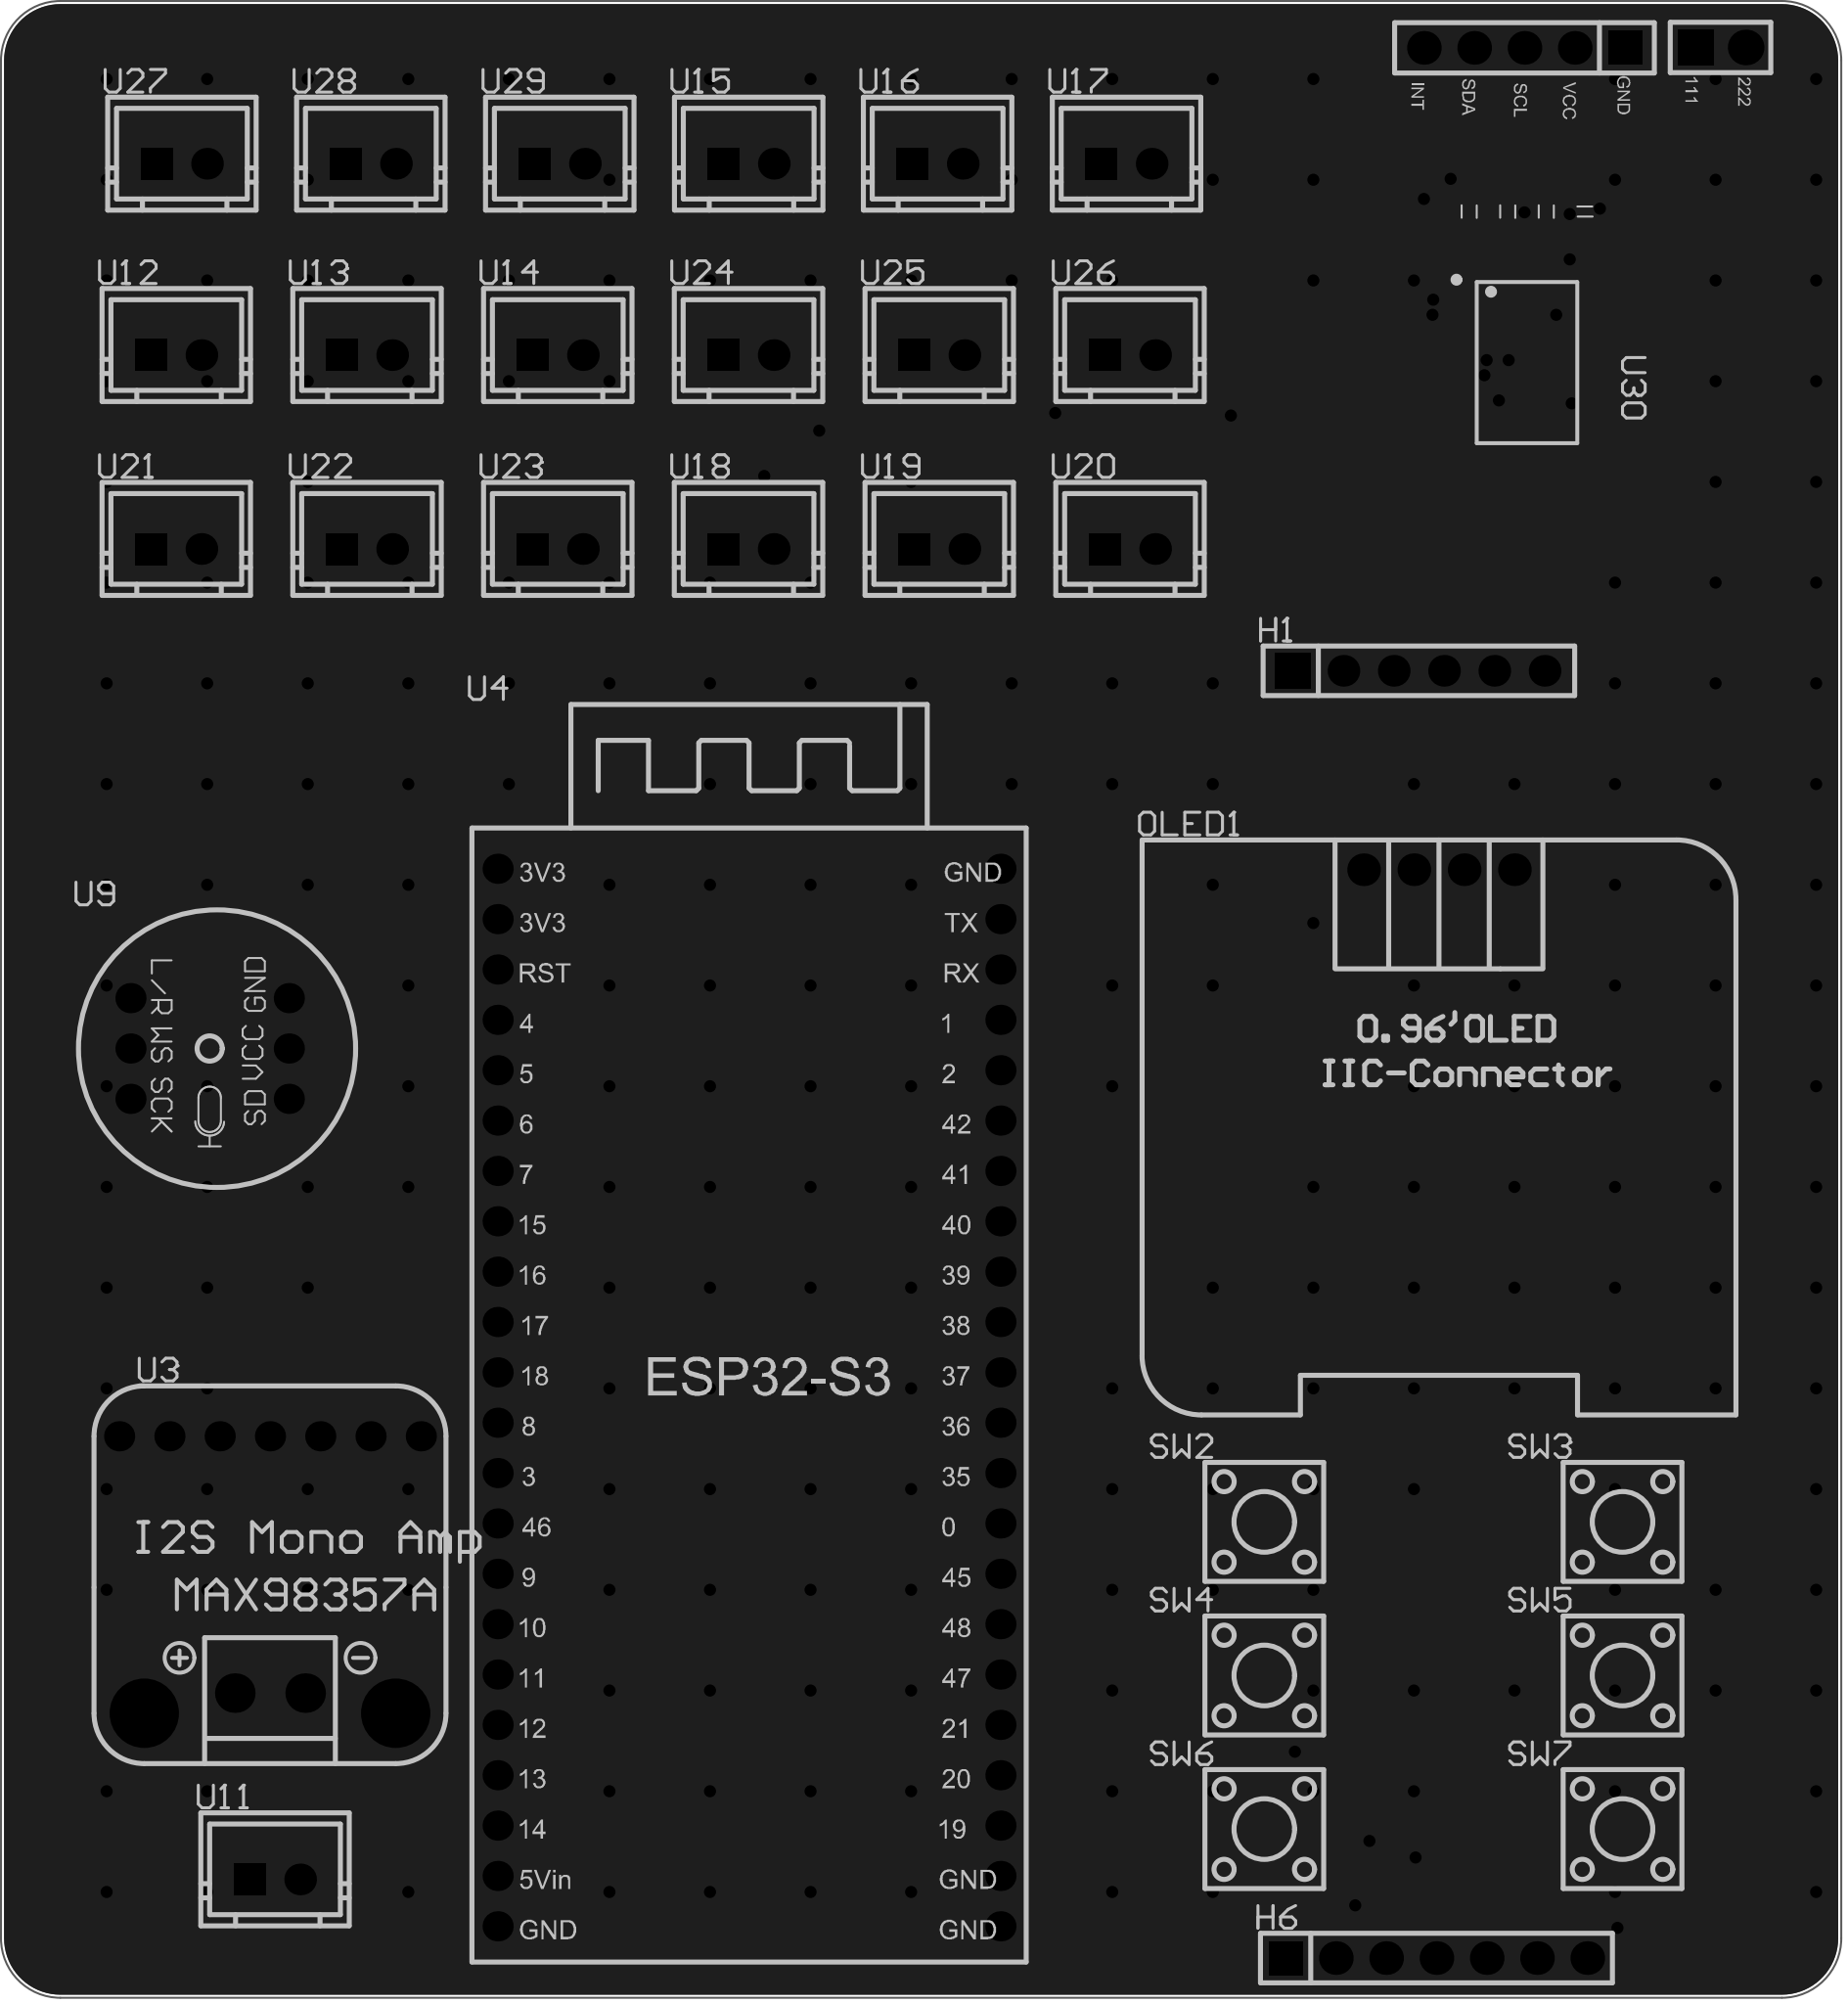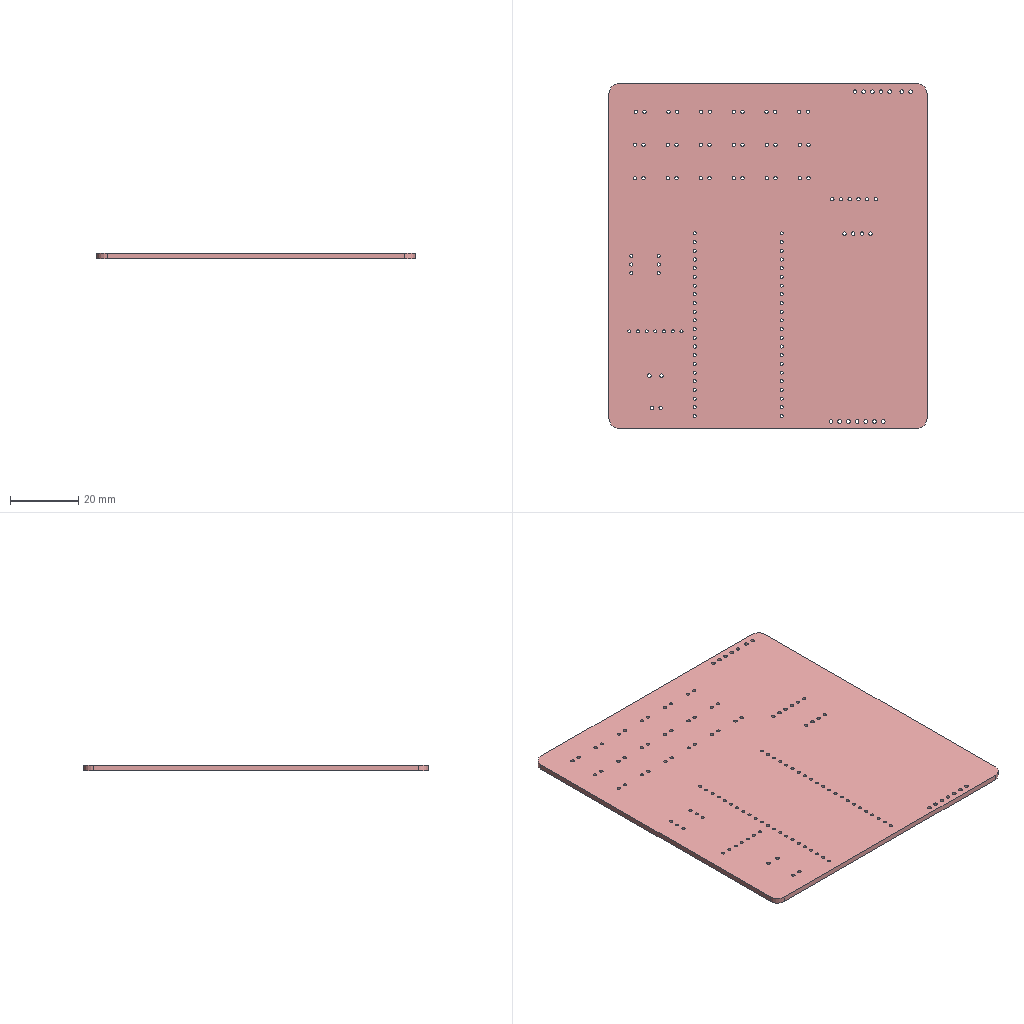Circuit board layout | Altium Designer | box 93 x 100.7 x 1.6 mm
Layer stack:
# Altium Designer layer stack of  (unit mm; dielectric type: 0 none, 1 core, 2 prepreg, 3 surface material)
index,name,kind,layer,copper_thickness_mm,dielectric_type,dielectric_thickness_mm,dielectric_material,dielectric_constant
0,Top Paste Mask Layer,other,,,,,,
1,Top Silkscreen Layer,other,,,,,,
2,Top Solder Mask Layer,dielectric,,,3,0.01,,3.3
3,Top Layer,copper,Top Layer,0.035,,,,
4,Dielectric1,dielectric,,,3,1.51,FR4,4.5
5,Bottom Layer,copper,Bottom Layer,0.035,,,,
6,Bottom Solder Mask Layer,dielectric,,,3,0.01,,3.3
7,Bottom Silkscreen Layer,other,,,,,,
8,Bottom Paste Mask Layer,other,,,,,,
# drill layer pairs: low layer,high layer
drill_pair,Top Layer,Bottom Layer
Part placement:
Designator,Comment,Layer,Footprint,Center-X(mm),Center-Y(mm),Rotation
OLED1,,TopLayer,0.96OLED_4P,154.432,139.827,0
SW2,KH-6X6X5H-STM,TopLayer,SW-SMD_4P-L6.0-W6.0-P4.50-LS9.0-2,145.606,106.934,0
SW3,KH-6X6X5H-STM,TopLayer,SW-SMD_4P-L6.0-W6.0-P4.50-LS9.0-2,163.703,106.934,0
SW4,KH-6X6X5H-STM,TopLayer,SW-SMD_4P-L6.0-W6.0-P4.50-LS9.0-2,145.606,99.187,0
SW5,KH-6X6X5H-STM,TopLayer,SW-SMD_4P-L6.0-W6.0-P4.50-LS9.0-2,163.703,99.187,0
SW6,KH-6X6X5H-STM,TopLayer,SW-SMD_4P-L6.0-W6.0-P4.50-LS9.0-2,145.606,91.44,0
SW7,KH-6X6X5H-STM,TopLayer,SW-SMD_4P-L6.0-W6.0-P4.50-LS9.0-2,163.703,91.44,0
U3,Adafruit MAX98357 I2S Amp,TopLayer,MAX98357_I2S_AMP_MODULE,95.377,104.775,270
U4,NO,TopLayer,ESP32S3,119.578,113.205,0
U9,INMP441,TopLayer,INMP441,92.329,130.81,0
U11,_x001F_XH2.54-2P,TopLayer,CONN-TH_2P-P2.54-V,95.631,88.9,0
U12,_x001F_XH2.54-2P,TopLayer,CONN-TH_2P-P2.54-V,90.643,165.783,0
U13,_x001F_XH2.54-2P,TopLayer,CONN-TH_2P-P2.54-V,100.279,165.783,0
U14,_x001F_XH2.54-2P,TopLayer,CONN-TH_2P-P2.54-V,109.915,165.783,0
U15,_x001F_XH2.54-2P,TopLayer,CONN-TH_2P-P2.54-V,119.559,175.435,0
U16,_x001F_XH2.54-2P,TopLayer,CONN-TH_2P-P2.54-V,129.103,175.435,0
U17,_x001F_XH2.54-2P,TopLayer,CONN-TH_2P-P2.54-V,138.647,175.435,0
U18,_x001F_XH2.54-2P,TopLayer,CONN-TH_2P-P2.54-V,119.55,156.005,0
U19,_x001F_XH2.54-2P,TopLayer,CONN-TH_2P-P2.54-V,129.186,156.005,0
U20,_x001F_XH2.54-2P,TopLayer,CONN-TH_2P-P2.54-V,138.822,156.005,0
U21,_x001F_XH2.54-2P,TopLayer,CONN-TH_2P-P2.54-V,90.643,156.005,0
U22,_x001F_XH2.54-2P,TopLayer,CONN-TH_2P-P2.54-V,100.279,156.005,0
U23,_x001F_XH2.54-2P,TopLayer,CONN-TH_2P-P2.54-V,109.915,156.005,0
U24,_x001F_XH2.54-2P,TopLayer,CONN-TH_2P-P2.54-V,119.55,165.783,0
U25,_x001F_XH2.54-2P,TopLayer,CONN-TH_2P-P2.54-V,129.186,165.783,0
U26,_x001F_XH2.54-2P,TopLayer,CONN-TH_2P-P2.54-V,138.822,165.783,0
U27,_x001F_XH2.54-2P,TopLayer,CONN-TH_2P-P2.54-V,90.927,175.435,0
U28,_x001F_XH2.54-2P,TopLayer,CONN-TH_2P-P2.54-V,100.471,175.435,0
U29,_x001F_XH2.54-2P,TopLayer,CONN-TH_2P-P2.54-V,110.015,175.435,0
C10,0.1uF,TopLayer,C0603-1,161.798,173.025,270
U30,PCF8575TS/1,112,TopLayer,SSOP-24_L8.2-W5.3-P0.65-LS7.8-BL,158.877,165.405,270
H4,KH-2.54PH180-1X5P-L11.5,TopLayer,HDR-TH_5P-P2.54-V-M,158.75,181.28,180
H1,,TopLayer,HDR-TH_6P-P2.54-V-F,153.416,149.86,0
R1,4.7K,TopLayer,R0603-1,157.903,173.025,90
R2,4.7K,TopLayer,R0603-1,155.956,173.025,90
R18,4.7K,TopLayer,R0603-1,159.851,173.025,90
H5,,TopLayer,HDR-TH_2P-P2.54-V-M-1,168.654,181.299,0
H6,,TopLayer,HDR-TH_7P-P2.54-V-M,154.302,84.933,0
Pad and via stacks:
# Altium Designer via and pad stacks of  (unit mm). Each distinct definition once, with the count of objects using it.
# via: kind,start_layer,end_layer,hole_mm,diameter_mm,mode(0 simple;1 top-mid-bottom;2 full stack),diameter_per_layer,count,example_net
# pad: kind,layer,hole_mm,hole_type(0 round;1 square;2 slot),plating,top_size,top_shape(1 round;2 rect;3 octagon;9 rounded rect),mid_size,bottom_size,mode,footprint,size_per_layer,count,example
pad,Multi-Layer,1,0,plated,1.65x1.65,1,1.65x1.65,1.65x1.65,0,0.96OLED_4P,,4,OLED1.4
pad,Multi-Layer,0.9144,0,plated,1.524x1.524,1,1.524x1.524,1.524x1.524,0,MAX98357 I2S AMP MODULE,,7,U3.1
pad,Multi-Layer,1.1,0,plated,2x2,1,2x2,2x2,0,MAX98357 I2S AMP MODULE,,2,U3.9
pad,Multi-Layer,0.9144,0,plated,1.524x1.524,1,1.524x1.524,1.524x1.524,0,ESP32S3,,44,U4.1
pad,Multi-Layer,0.9144,0,plated,1.524x1.524,1,1.524x1.524,1.524x1.524,0,INMP441,,6,U9.5
pad,Multi-Layer,1,0,plated,1.6x1.6,1,1.6x1.6,1.6x1.6,0,CONN-TH_2P-P2.54-V,,19,U11.2
pad,Multi-Layer,1,0,plated,1.6x1.6,2,1.6x1.6,1.6x1.6,0,CONN-TH_2P-P2.54-V,,19,U11.1
pad,Multi-Layer,1.1,0,plated,1.7x1.7,2,1.7x1.7,1.7x1.7,0,HDR-TH_5P-P2.54-V-M,,1,H4.1
pad,Multi-Layer,1.1,0,plated,1.7x1.7,1,1.7x1.7,1.7x1.7,0,HDR-TH_5P-P2.54-V-M,,4,H4.2
pad,Multi-Layer,1.02,0,plated,1.6x1.6,1,1.6x1.6,1.6x1.6,0,HDR-TH_6P-P2.54-V-F,,5,H1.6
pad,Multi-Layer,1.02,0,plated,1.8x1.8,2,1.8x1.8,1.8x1.8,0,HDR-TH_6P-P2.54-V-F,,1,H1.1
pad,Multi-Layer,1.1,0,plated,1.8x1.8,1,1.8x1.8,1.8x1.8,0,HDR-TH_2P-P2.54-V-M-1,,1,H5.2
pad,Multi-Layer,1.1,0,plated,1.8x1.8,2,1.8x1.8,1.8x1.8,0,HDR-TH_2P-P2.54-V-M-1,,1,H5.1
pad,Multi-Layer,1.1,0,plated,1.7x1.7,2,1.7x1.7,1.7x1.7,0,HDR-TH_7P-P2.54-V-M,,1,H6.1
pad,Multi-Layer,1.1,0,plated,1.7x1.7,1,1.7x1.7,1.7x1.7,0,HDR-TH_7P-P2.54-V-M,,6,H6.2
pad,Top Layer,0,0,plated,2.3x1.5,2,2.3x1.5,2.3x1.5,0,SW-SMD_4P-L6.0-W6.0-P4.50-LS9.0-2,,24,SW2.1
pad,Top Layer,0,0,plated,0.635x0.9799,2,0.635x0.9799,0.635x0.9799,0,C0603-1,,2,C10.1
pad,Top Layer,0,0,plated,0.4x1.5,1,0.4x1.5,0.4x1.5,0,SSOP-24_L8.2-W5.3-P0.65-LS7.8-BL,,24,U30.1
pad,Top Layer,0,0,plated,0.635x0.9799,2,0.635x0.9799,0.635x0.9799,0,R0603-1,,6,R1.2
via,Top Layer,Bottom Layer,0.3048,0.6096,0,,261,$1N6804
via,Top Layer,Bottom Layer,2.499,3.5,0,,2,
Copper pours:
name,layer,net,type(0 solid;1 hatched;2 none)
Top Layer-GND,Top Layer,GND,0
Bottom Layer-GND,Bottom Layer,GND,0
Design rules, without the lines most boards share:
# Altium Designer design rules of  (exported by Altium Designer, unit mm)
# columns: name | kind | enabled | priority | scope1 | scope2 | descriptor | typed fields (field=value)
Plane_Default | 0 | disabled | 1 | All | All | Clearance Constraint (Gap=6mil) (Disabled)(All),(All) | gap=0.1524
Plane_Default_1 | 63 | disabled | 1 | All | All | Board Clearance Constraint (Gap=0mil) (Disabled)(All) |
Copper_Default | 0 | disabled | 2 | All | All | Clearance Constraint (Gap=6mil) (Disabled)(All),(All) | gap=0.1524
Copper_Default_1 | 63 | disabled | 2 | All | All | Board Clearance Constraint (Gap=0mil) (Disabled)(All) |
Copper_gge24019 | 0 | disabled | 3 | All | All | Clearance Constraint (Gap=6mil) (Disabled)(All),(All) | gap=0.1524
Copper_gge24019_1 | 63 | disabled | 3 | All | All | Board Clearance Constraint (Gap=0mil) (Disabled)(All) |
Default | 0 | enabled | 4 | All | All | Clearance Constraint (Gap=6mil) (All),(All) | gap=0.1524
Default_1 | 63 | enabled | 4 | All | All | Board Clearance Constraint (Gap=0mil) (All) |
otherClearance | 52 | enabled | 1 | All | All | Hole To Hole Clearance (Gap=11.8mil) (All),(All) | gap=0.2997
Default_2 | 2 | enabled | 1 | All | All | Width Constraint (Min=10mil) (Max=1000mil) (Preferred=30mil) (All) |
Default_3 | 11 | enabled | 1 | All | All | Routing Via (MinHoleWidth=12mil) (MaxHoleWidth=2362mil) (PreferredHoleWidth=12mil) (MinWidth=24mil) (MaxWidth=3938mil) (PreferedWidth=24mil) (All) | via_min_hole=0.3048 via_max_hole=59.995 via_preferred_diameter=0.6096 via_preferred_hole=0.3048
Default_4 | 6 | enabled | 1 | All | All | Power Plane Connect Rule(Relief Connect )(Expansion=20mil) (Conductor Width=0mil) (Air Gap=10mil) (Entries=4) (All) | relief_conductor_width=0 relief_entries=4 relief_expansion=0.508
gge24019 | 20 | disabled | 1 | All | All | Polygon Connect Rule(Relief Connect )(Conductor Width=0mil) (Relief Angle=90 Angle) (Entries=4) (Air Gap Width=1mil) (Disabled)(All),(All) | connect_style(0=relief,1=direct,2=none)=0 relief_conductor_width=0 relief_entries=4
Default_5 | 20 | enabled | 2 | All | All | Polygon Connect Rule(Relief Connect )(Conductor Width=0mil) (Relief Angle=90 Angle) (Entries=4) (Air Gap Width=1mil) (All),(All) | connect_style(0=relief,1=direct,2=none)=0 relief_conductor_width=0 relief_entries=4
Common | 14 | enabled | 1 | All | All | Paste Mask Expansion (Expansion =0mil) (All) | expansion=0
Common_1 | 13 | enabled | 2 | All | All | Solder Mask Expansion (Expansion =2mil) (All) | expansion=0.0508
Common_2 | 13 | enabled | 1 | IsVia | All | Solder Mask Expansion (Expansion =-1000mil) (IsVia) | expansion=-25.4